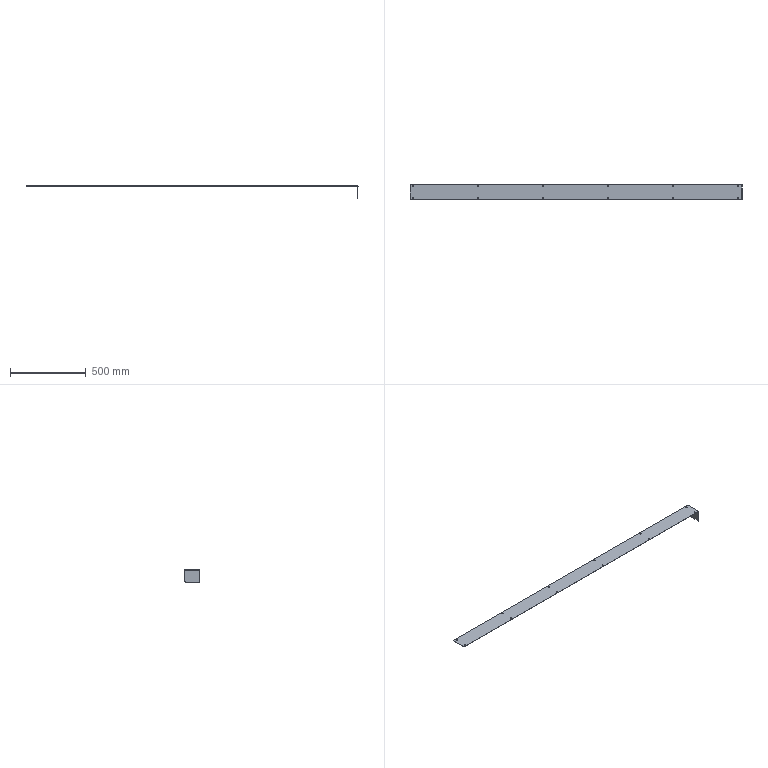Part | SolidWorks | features Fillet 1, FlatPattern 1, ICE 1, LPattern 1, SMBaseFlange 1, SMMiteredFlange 1, SheetMetal 1 | 1 solid | 68 faces | box 2196 x 100 x 80 mm | volume 339571 mm3 | plane 37 | cylinder 31 | commonest cylinder face diameters 6 x24 4 x5 2 x1 5 x1